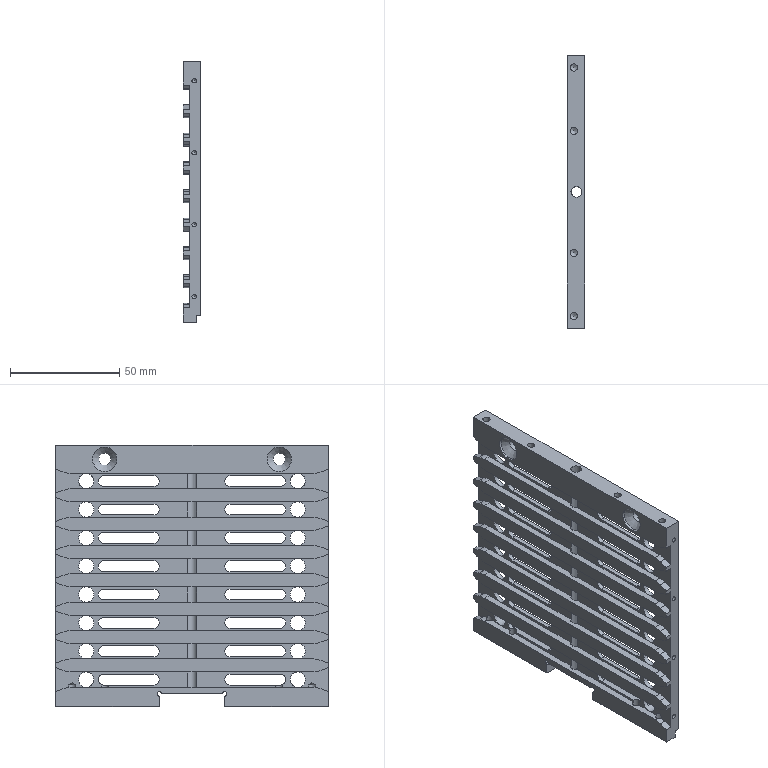CAM job | NX | 3+2 milling, drilling | part box 8 x 125 x 120 mm | stock box 10 x 130 x 125 mm
Tools:
number,name,description,diameter,corner_radius,flute_length,length,flutes
4,D4,平底铣刀-粗,4.0,0.0,25.0,75.0,2
6,D6,平底铣刀-粗,6.0,0.0,25.0,75.0,2
9,D10,平底铣刀-粗,10.0,0.0,35.0,75.0,2
20,D2-J,平底铣刀-精,2.0,0.0,50.0,75.0,2
11,D4-J,平底铣刀-精,4.0,0.0,50.0,75.0,2
7,D6-J,平底铣刀-精,6.0,0.0,25.0,75.0,2
1,D80R0.8FACEMILL,圆鼻刀-粗,80.0,0.8,50.0,75.0,2
1,D80R0.8FACEMILL-J,圆鼻刀-精,80.0,0.8,50.0,75.0,2
2,D6CHAMFERMILL,倒角刀,6.0,0.0,3.0,25.0,2
19,ZT2,钻头,2.0,0.0,35.0,50.0,2
17,ZT5.5,钻头,5.5,0.0,35.0,50.0,2
18,ZT7,钻头,7.0,0.0,35.0,50.0,2
Operations:
program,operation,operation_type,tool,method,geometry_group,spindle_rpm,surface_speed,feed_per_tooth,feed_cut,feed_plunge,cut_length_mm,path_length_mm,cut_time_min,machine_time_min
A,TOPFACE,FaceMilling,D80R0.8FACEMILL,SIDEFINISH-DEPTHK-STEPG,W-A,4500.0,1385.0,0.1667,1500.0,100.0,729.0,785.0,0.486,0.4916
A,OUTLINEROUGH_2,VolumeBased25DMillingOperation,D10,METHOD,W-A,8000.0,251.327,0.375,6000.0,80.0,6357.503,6424.003,1.06,1.066
A,FLOORWALLROUGH_1,VolumeBased25DMillingOperation,D10,METHOD,W-A,9000.0,282.743,0.2222,4000.0,100.0,8953.464,9430.477,2.238,2.286
A,SPOTDRILL,Operation,D6CHAMFERMILL,METHOD,W-A,3000.0,56.0,0.0333,200.0,0.0,5.1,101.217,0.0255,0.0351
A,SPOTDRILL-DEPTH0.8,Operation,D6CHAMFERMILL,NONE,W-A,8000.0,150.796,0.0312,500.0,90.0,25.2,389.237,0.0504,0.0868
A,PREDRILL3,Operation,ZT2,METHOD,W-A,3800.0,33.0,0.0132,100.0,0.0,22.0,135.017,0.22,0.2313
A,THROUGHHOLE-5-6,Operation,ZT5.5,NONE,W-A,3000.0,51.836,0.025,150.0,90.0,25.305,191.616,0.1687,0.1853
A,THROUGHHOLE-6-8,Operation,ZT7,NONE,W-A,2500.0,54.978,0.03,150.0,90.0,85.236,474.861,0.5682,0.6072
A,THROUGHSLOTROUGH_1,VolumeBased25DMillingOperation,D4,METHOD,W-A,12000.0,150.796,0.0333,800.0,100.0,14283.968,15435.789,17.855,17.97
A,THROUGHSLOTROUGH_1_COPY,VolumeBased25DMillingOperation,D4,METHOD,W-A,12000.0,150.796,0.0333,800.0,100.0,3981.107,4166.613,4.976,4.995
A,FLOORHELICALROUGHSMALL_COPY,VolumeBased25DMillingOperation,D4,LAYEREDROUGH-DEPTHK-STEPG,W-A,8000.0,100.531,0.0813,1300.0,100.0,1148.261,2186.533,0.8833,0.9871
A,FLOORHELICALROUGHSMALL_COPY_COPY,VolumeBased25DMillingOperation,D4,LAYEREDROUGH-DEPTHK-STEPG,W-A,8000.0,100.531,0.0813,1300.0,100.0,734.816,1269.38,0.5652,0.6187
A,FLOORFINISH_1,VolumeBased25DMillingOperation,D6-J,METHOD,W-A,9000.0,169.646,0.0833,1500.0,100.0,2295.827,2506.126,1.531,1.552
A,FLOORSIDEFINISH_3,VolumeBased25DMillingOperation,D6-J,METHOD,W-A,9000.0,169.646,0.0556,1000.0,100.0,528.192,754.435,0.5282,0.5508
A,FLOORSIDEFINISH_4,VolumeBased25DMillingOperation,D6-J,METHOD,W-A,9000.0,169.646,0.0667,1200.0,100.0,114.483,263.083,0.0954,0.1103
A,SLOTFINISH_1,VolumeBased25DMillingOperation,D4-J,METHOD,W-A,8000.0,100.531,0.0312,500.0,100.0,719.179,1953.772,1.438,1.562
A,SLOTFINISH_1_COPY,VolumeBased25DMillingOperation,D4-J,METHOD,W-A,8000.0,100.531,0.0312,500.0,100.0,205.48,415.38,0.411,0.4319
A,FLOORHELICALFINISHSMALL_COPY,VolumeBased25DMillingOperation,D4-J,HELICALFINISH-DEPTHK-STEPG,W-A,8000.0,100.528,0.05,800.0,100.0,362.056,1380.939,0.4526,0.5545
A,FLOORHELICALFINISHSMALL_COPY_COPY,VolumeBased25DMillingOperation,D4-J,HELICALFINISH-DEPTHK-STEPG,W-A,8000.0,100.528,0.05,800.0,100.0,197.011,735.923,0.2463,0.3002
A,CONTOURSMOOTHCORNERD2REF6_COPY,ZLevelMilling,D2-J,LAYEREDFINISH-DEPTHK-STEPG,W-A,8000.0,50.264,0.05,800.0,100.0,2061.061,2162.847,2.576,2.587
A,SELECTEDBODYONLY,SurfaceContour,D6CHAMFERMILL,METHOD,W-A,8000.0,150.796,0.1875,3000.0,100.0,2086.044,4787.588,0.6953,0.9655
A,MILLCHAMFER_1,PlanarMilling,D6CHAMFERMILL,METHOD,W-A,8000.0,150.796,0.0312,500.0,100.0,39.377,243.348,0.0788,0.0992
A,MILLCHAMFER_2,PlanarMilling,D6CHAMFERMILL,METHOD,W-A,8000.0,150.796,0.05,800.0,100.0,286.984,1318.401,0.3587,0.4619
A,OUTLINESEMIFINISH_2,VolumeBased25DMillingOperation,D6-J,METHOD,W-A,9000.0,169.646,0.0667,1200.0,100.0,523.191,598.191,0.436,0.4435
B,FLOORFACEMILLROUGH_COPY,VolumeBased25DMillingOperation,D80R0.8FACEMILL,LAYEREDROUGH-DEPTHK-STEPG,W-B,4500.0,1130.973,0.2222,2000.0,100.0,2740.097,3538.928,1.37,1.45
B,FLOORFACEMILLFINISH_COPY,VolumeBased25DMillingOperation,D80R0.8FACEMILL-J,SIDEFINISH-DEPTHK-STEPG,W-B,4500.0,1130.973,0.1111,1000.0,100.0,684.241,780.241,0.6842,0.6938
B,FLOORLAYEREDROUGHMID_COPY,VolumeBased25DMillingOperation,D6,LAYEREDROUGH-DEPTHK-STEPG,W-B,8000.0,150.792,0.1875,3000.0,100.0,13742.886,13933.879,4.581,4.6
B,CONTOURHELICALWALL_COPY,ZLevelMilling,D4-J,CONTOURWALL-DEPTHK-STEPG,W-B,7000.0,87.965,0.1071,1500.0,100.0,10423.196,10701.363,6.949,6.977
B,PLANEDEBURR6X45L_COPY,SurfaceContour,D6CHAMFERMILL,WALLCHAMFER-DEPTH0-STEPG,W-B,6500.0,122.519,0.1154,1500.0,100.0,2559.742,3660.635,1.706,1.817
B,FLOORCHAMFER_COPY,VolumeBased25DMillingOperation,D6CHAMFERMILL,WALLCHAMFER-DEPTH0-STEPG,W-B,6500.0,122.519,0.1154,1500.0,100.0,119.592,450.118,0.0797,0.1128
B,CONTOURFINISHMID_COPY,ZLevelMilling,D6-J,SIDEFINISH-DEPTHK-STEPG,W-B,8000.0,150.792,0.0625,1000.0,100.0,2123.966,2859.179,2.124,2.197